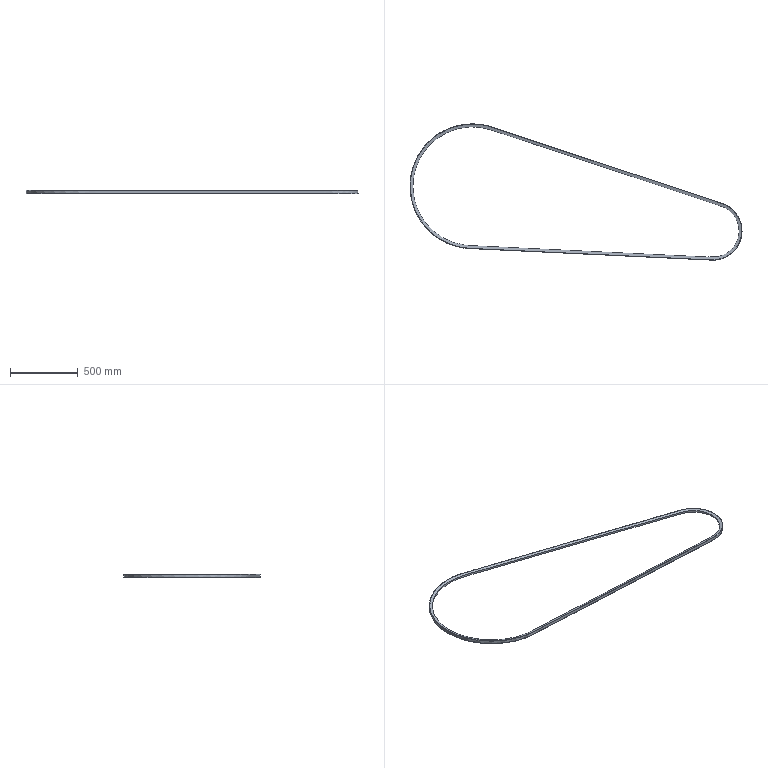Part | NX | features DATUM_CSYS 1, LINKED_BODY 1 | 1 solid | 6 faces | box 2447 x 1004 x 24.054 mm | volume 1773043 mm3 | spline 6